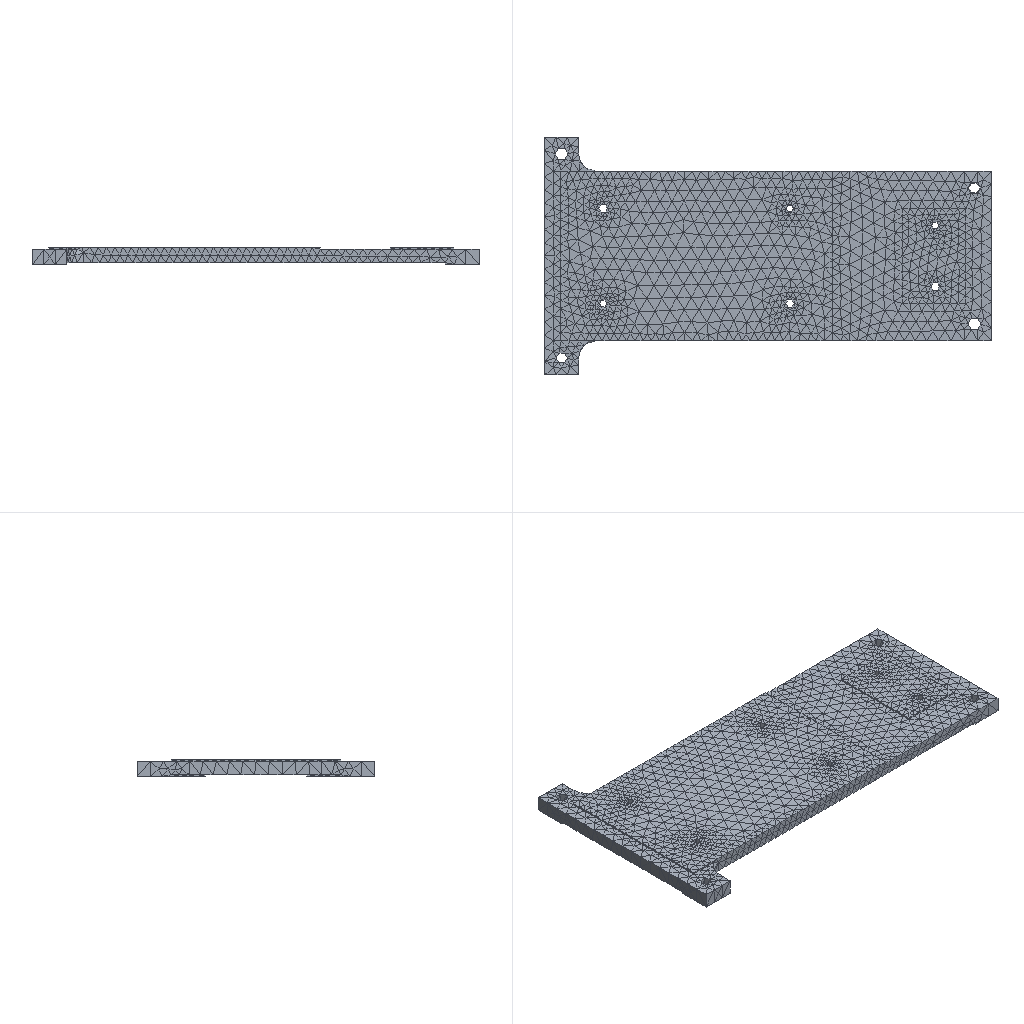Simulation study | nx simcenter
Set-up summary:
category,name,step,type,value,unit,region
solver,nx_nastran (Simcenter)
units,not stated in the deck,,not stated
analysis,deck,,static,static
analysis,solution,,SOL,101
load_step,SUBCASE 1,1,SUBCASE,SPC=1 LOAD=101
load_step,requested,,,1
mesh,nodes,,,15025
mesh,elements,,,7810
element_type,CTETRA,,solid,7810
load,nodal force total,,FX,0.0,model units
load,nodal force total,,FY,0.0,model units
load,nodal force total,,FZ,-50000,model units
load,load commands in deck,,count,2058
load,GRAV,,command,1
bc,support commands in deck,,count,366
analysis,NX solution 0,,Structural,Linear Statics - Single Constraint
check,setup vs results,,match,every grid point's frame and coordinates and every element id; grid points of CTETRA elements
Nastran input file, long lists of numbers shortened:
$*$$$$$$$$$$$$$$$$$$$$$$$$$$$$$$$$$$$$$$$$$$$$$$$$$$$$$$$$$$$$$$$$$
$*
$*                    NX v10.0.0.24 TRANSLATOR
$*                    FOR NX NASTRAN VERSION 10.0
$ (33 more lines like these left out)
ASSIGN OUTPUT2='1_sim1-1.op2' UNIT=12
$*
$*$$$$$$$$$$$$$$$$$$$$$$$$$$$$$$$$$$$
$*
$* EXECUTIVE CONTROL
$*
$*$$$$$$$$$$$$$$$$$$$$$$$$$$$$$$$$$$$
$*
ID,NASTRAN,1_sim1-1
SOL 101
CEND
$*
$*$$$$$$$$$$$$$$$$$$$$$$$$$$$$$$$$$$$
$*
$* CASE CONTROL
$*
$*$$$$$$$$$$$$$$$$$$$$$$$$$$$$$$$$$$$
$*
TITLE = 1
ECHO = NONE
SPC = 1
OUTPUT
BCRESULTS(TRACTION,FORCE,PLOT) = ALL
DISPLACEMENT(PLOT) = ALL
ESE(PLOT) = ALL
FORCE(PLOT,CORNER) = ALL
OLOAD(PLOT) = ALL
SPCFORCES(PLOT) = ALL
STRAIN(PLOT,FIBER,CORNER) = ALL
STRESS(PLOT,CORNER) = ALL
$*  NX Step: Subcase - Static Loads 1
SUBCASE 1
LABEL = Subcase - Static Loads 1
LOAD = 101
$*
$*$$$$$$$$$$$$$$$$$$$$$$$$$$$$$$$$$$$
$*
$* BULK DATA
$*
$*$$$$$$$$$$$$$$$$$$$$$$$$$$$$$$$$$$$
$*
BEGIN BULK
$*
$* PARAM CARDS
$*
PARAM      K6ROT100.0000
PARAM     OIBULK     YES
PARAM    OMACHPR     YES
PARAM       POST      -2
PARAM    POSTEXT     YES
PARAM    UNITSYS   MN-MM
$*
$* GRID CARDS
$*
GRID*              14950               0-6.304916000E+01-1.980000000E+02+
*       -9.000000000E+00               0
GRID*              14951               0-6.304916000E+01-1.980000000E+02+
*       0.0000000000E+00               0
$ (30046 more lines like these left out)
$*
$* ELEMENT CARDS
$*
$*  NX Mesh Collector: Solid(1)
$*  NX Mesh: 3d_mesh(1)
CTETRA         1       1       1       2       3       4     307     308+
+            309     310     311     312
CTETRA         2       1       4       5       1   14338     313     314+
+            310     315     316     317
$ (15616 more lines like these left out)
$*
$* PROPERTY CARDS
$*
$*  NX Property: PSOLID1
PSOLID         1       1       0                           SMECH
$*
$* MATERIAL CARDS
$*
$*  NX Material: Aluminum_6061
MAT1           16.8980+7        0.3300002.7110-62.2161-5
MATT1          1       1               2               3
TABLEM1        1                                                        +
+        20.00006.8980+7 21.11006.8980+7 23.89006.8980+7 37.78006.8290+7+
+        51.67006.8290+7 65.56006.7600+7 79.44006.6910+7 93.33006.6221+7+
+       107.22006.5531+7121.11006.4841+7135.00006.4151+7148.89006.3461+7+
+       162.78006.2772+7176.67006.1392+7190.56006.0702+7204.44005.9323+7+
+       218.33005.8633+7232.22005.7253+7246.11005.5874+7260.00005.4494+7+
+       273.89005.3114+7287.78005.1735+7301.67005.0355+7315.56004.8976+7+
+       329.44004.7596+7343.33004.6216+7357.22004.4147+7371.11004.2767+7+
+       385.00004.1388+7398.89003.9318+7412.78003.7939+7426.67003.5869+7+
+           ENDT
TABLEM1        2                                                        +
+        20.00000.330000 21.11000.330000    ENDT
TABLEM1        3                                                        +
+        20.00002.2380-5 93.33002.3184-5107.22002.3346-5121.11002.3508-5+
+       135.00002.3670-5148.89002.3832-5162.78002.3994-5176.67002.4138-5+
+       190.56002.4300-5204.44002.4444-5218.33002.4588-5232.22002.4732-5+
+       246.11002.4876-5260.00002.5002-5273.89002.5146-5287.78002.5272-5+
+       301.67002.5398-5315.56002.5524-5    ENDT
$*
$* LOAD AND CONSTRAINT CARDS
$*
$*  NX Load and Constraint: Fixed(1)
SPC            1    6344  123456  0.0000
SPC            1    6345  123456  0.0000
SPC            1    6346  123456  0.0000
SPC            1    6347  123456  0.0000
$ (362 more lines like these left out)
$*  NX Load and Constraint: Force(1)
FORCE          2    7265       0 16.2699  0.0000  0.0000-1.00000
FORCE          2    7266       0 13.9042  0.0000  0.0000-1.00000
FORCE          2    7267       08.935865  0.0000  0.0000-1.00000
FORCE          2    7268       0 13.9569  0.0000  0.0000-1.00000
$ (2053 more lines like these left out)
$*  NX Load and Constraint: Gravity(1)
GRAV           3       0 9810.00  0.0000  0.0000-1.00000
LOAD         1011.0000001.000000       21.000000       3
ENDDATA e993327d
Results summary:
result,analysis,,,static
result,last_loadstep,,,1
result,primary field,,,displacements
result,reaction total,,FX,-0.005234,model units
result,reaction total,,FY,0.003058,model units
result,reaction total,,FZ,56241.594,model units
result,NX solution 0,,loadcases,1,mm